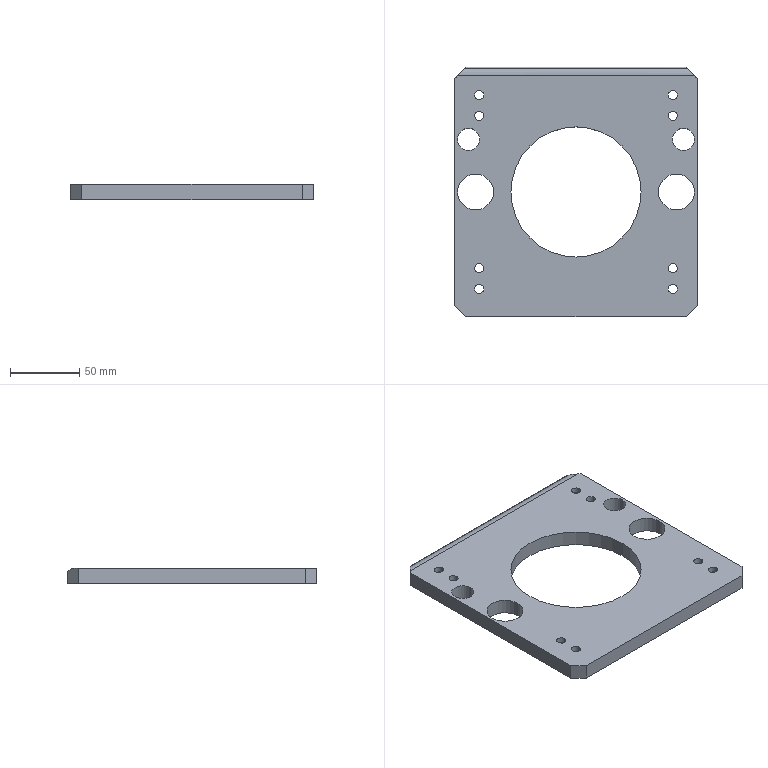Part | STEP file | PN_0025 Snap-ring height stop block | 1 solid | 62 faces | box 175 x 180 x 11 mm | volume 245670 mm3 | cylinder 43 | plane 19 | commonest cylinder face diameters 6.6 x16 11 x16 16 x4 26 x4 94 x2 20 x1